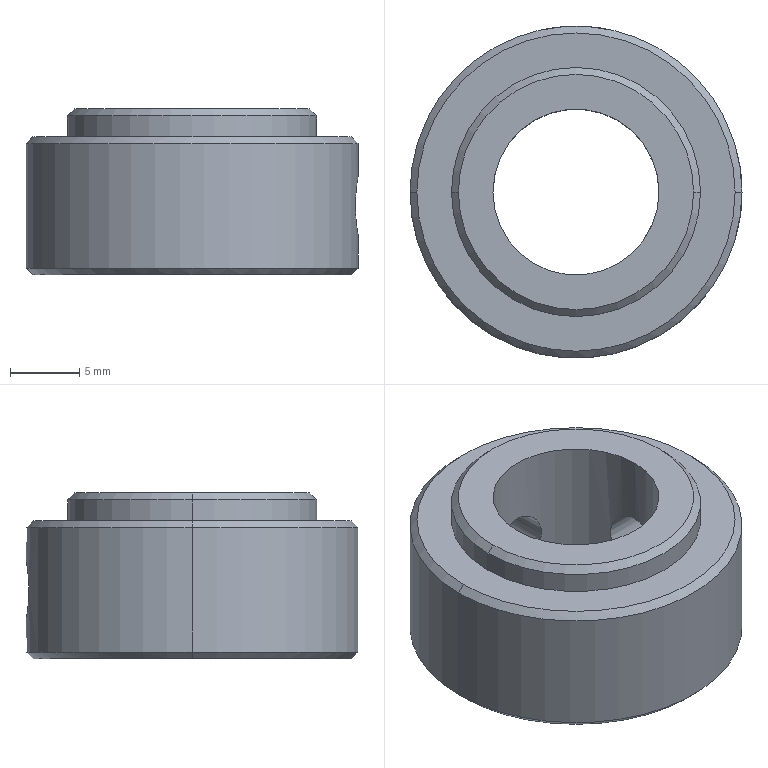Part | STEP file | 2011 Stopper shaft | 1 solid | 19 faces | box 24 x 24 x 12 mm | volume 3483 mm3 | cylinder 10 | cone 6 | plane 3 | commonest cylinder face diameters 4.2 x4 12 x2 18 x2 24 x2